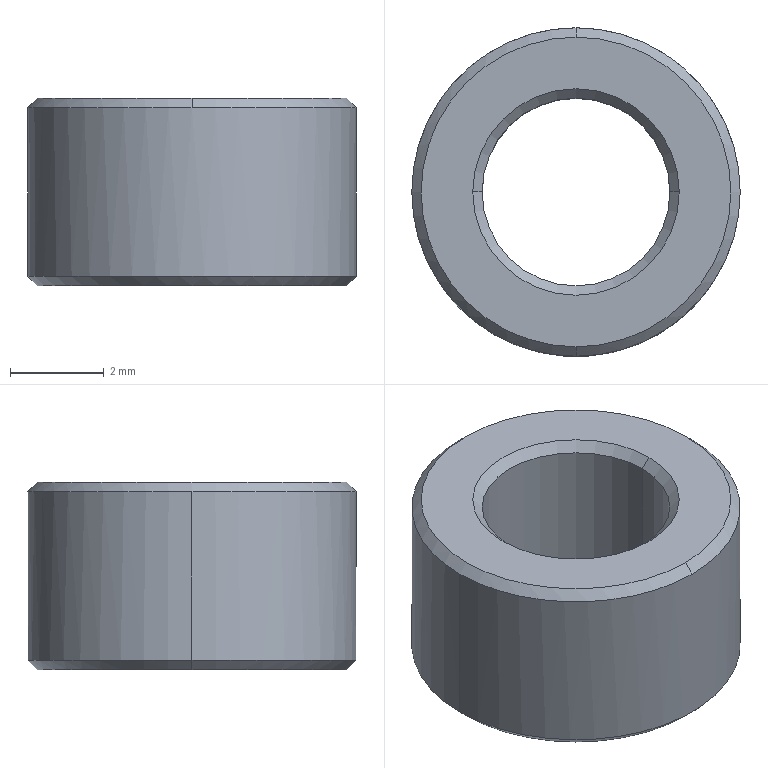Part | STEP file | 0243_001_FWSSM-D7-V4-T4 | 1 solid | 14 faces | box 7 x 7 x 4 mm | volume 102.29 mm3 | cone 8 | cylinder 4 | plane 2 | commonest cylinder face diameters 4 x2 7 x2
STEP:
#1=CARTESIAN_POINT('',(0.,0.,0.));
#2=DIRECTION('',(0.,0.,1.));
#3=DIRECTION('',(1.,0.,0.));
#4=AXIS2_PLACEMENT_3D('',#1,#2,#3);
#5=CARTESIAN_POINT('',(3.5,0.,-3.8));
#6=VERTEX_POINT('',#5);
#7=CARTESIAN_POINT('',(-3.5,0.,-3.8));
#8=VERTEX_POINT('',#7);
#9=CARTESIAN_POINT('',(0.,0.,-3.8));
#10=DIRECTION('',(0.,0.,1.));
#11=DIRECTION('',(1.,0.,0.));
#12=AXIS2_PLACEMENT_3D('',#9,#10,#11);
#13=CIRCLE('',#12,3.5);
#14=CARTESIAN_POINT('',(0.,0.,-2.));
#15=DIRECTION('',(0.,0.,1.));
#16=DIRECTION('',(1.,0.,0.));
#17=AXIS2_PLACEMENT_3D('',#14,#15,#16);
#18=CYLINDRICAL_SURFACE('',#17,3.5);
#19=CARTESIAN_POINT('',(0.,-1.8));
#20=DIRECTION('',(1.,0.));
#21=VECTOR('',#20,1.);
#22=LINE('',#19,#21);
#23=(GEOMETRIC_REPRESENTATION_CONTEXT(2)PARAMETRIC_REPRESENTATION_CONTEXT()REPRESENTATION_CONTEXT('',''));
#24=DEFINITIONAL_REPRESENTATION('',(#22),#23);
#25=PCURVE('',#18,#24);
#26=CARTESIAN_POINT('',(0.,0.,-3.8));
#27=DIRECTION('',(0.,0.,1.));
#28=DIRECTION('',(1.,0.,0.));
#29=AXIS2_PLACEMENT_3D('',#26,#27,#28);
#30=CONICAL_SURFACE('',#29,3.5,0.7854);
#31=CARTESIAN_POINT('',(0.,0.));
#32=DIRECTION('',(1.,0.));
#33=VECTOR('',#32,1.);
#34=LINE('',#31,#33);
#35=(GEOMETRIC_REPRESENTATION_CONTEXT(2)PARAMETRIC_REPRESENTATION_CONTEXT()REPRESENTATION_CONTEXT('',''));
#36=DEFINITIONAL_REPRESENTATION('',(#34),#35);
#37=PCURVE('',#30,#36);
#38=SURFACE_CURVE('',#13,(#25,#37),.PCURVE_S1.);
#39=EDGE_CURVE('',#6,#8,#38,.T.);
#40=ORIENTED_EDGE('',*,*,#39,.T.);
#41=CARTESIAN_POINT('',(-3.5,0.,-0.2));
#42=VERTEX_POINT('',#41);
#43=CARTESIAN_POINT('',(-3.5,0.,-2.));
#44=DIRECTION('',(0.,0.,1.));
#45=VECTOR('',#44,1.);
#46=LINE('',#43,#45);
#47=CARTESIAN_POINT('',(3.142,0.));
#48=DIRECTION('',(0.,1.));
#49=VECTOR('',#48,1.);
#50=LINE('',#47,#49);
#51=(GEOMETRIC_REPRESENTATION_CONTEXT(2)PARAMETRIC_REPRESENTATION_CONTEXT()REPRESENTATION_CONTEXT('',''));
#52=DEFINITIONAL_REPRESENTATION('',(#50),#51);
#53=PCURVE('',#18,#52);
#54=CARTESIAN_POINT('',(0.,0.,-2.));
#55=DIRECTION('',(0.,0.,1.));
#56=DIRECTION('',(1.,0.,0.));
#57=AXIS2_PLACEMENT_3D('',#54,#55,#56);
#58=CYLINDRICAL_SURFACE('',#57,3.5);
#59=CARTESIAN_POINT('',(3.142,0.));
#60=DIRECTION('',(0.,1.));
#61=VECTOR('',#60,1.);
#62=LINE('',#59,#61);
#63=(GEOMETRIC_REPRESENTATION_CONTEXT(2)PARAMETRIC_REPRESENTATION_CONTEXT()REPRESENTATION_CONTEXT('',''));
#64=DEFINITIONAL_REPRESENTATION('',(#62),#63);
#65=PCURVE('',#58,#64);
#66=SURFACE_CURVE('',#46,(#53,#65),.PCURVE_S1.);
#67=EDGE_CURVE('',#8,#42,#66,.T.);
#68=ORIENTED_EDGE('',*,*,#67,.T.);
#69=CARTESIAN_POINT('',(0.,3.5,-0.2));
#70=VERTEX_POINT('',#69);
#71=CARTESIAN_POINT('',(0.,0.,-0.2));
#72=DIRECTION('',(0.,0.,-1.));
#73=DIRECTION('',(1.,0.,0.));
#74=AXIS2_PLACEMENT_3D('',#71,#72,#73);
#75=CIRCLE('',#74,3.5);
#76=CARTESIAN_POINT('',(6.283,1.8));
#77=DIRECTION('',(-1.,0.));
#78=VECTOR('',#77,1.);
#79=LINE('',#76,#78);
#80=(GEOMETRIC_REPRESENTATION_CONTEXT(2)PARAMETRIC_REPRESENTATION_CONTEXT()REPRESENTATION_CONTEXT('',''));
#81=DEFINITIONAL_REPRESENTATION('',(#79),#80);
#82=PCURVE('',#18,#81);
#83=CARTESIAN_POINT('',(0.,0.,-0.2));
#84=DIRECTION('',(0.,0.,-1.));
#85=DIRECTION('',(0.,1.,0.));
#86=AXIS2_PLACEMENT_3D('',#83,#84,#85);
#87=CONICAL_SURFACE('',#86,3.5,0.7854);
#88=CARTESIAN_POINT('',(1.571,0.));
#89=DIRECTION('',(1.,0.));
#90=VECTOR('',#89,1.);
#91=LINE('',#88,#90);
#92=(GEOMETRIC_REPRESENTATION_CONTEXT(2)PARAMETRIC_REPRESENTATION_CONTEXT()REPRESENTATION_CONTEXT('',''));
#93=DEFINITIONAL_REPRESENTATION('',(#91),#92);
#94=PCURVE('',#87,#93);
#95=SURFACE_CURVE('',#75,(#82,#94),.PCURVE_S1.);
#96=EDGE_CURVE('',#42,#70,#95,.T.);
#97=ORIENTED_EDGE('',*,*,#96,.T.);
#98=CARTESIAN_POINT('',(3.5,0.,-0.2));
#99=VERTEX_POINT('',#98);
#100=CARTESIAN_POINT('',(0.,0.,-0.2));
#101=DIRECTION('',(0.,0.,-1.));
#102=DIRECTION('',(1.,0.,0.));
#103=AXIS2_PLACEMENT_3D('',#100,#101,#102);
#104=CIRCLE('',#103,3.5);
#105=CARTESIAN_POINT('',(6.283,1.8));
#106=DIRECTION('',(-1.,0.));
#107=VECTOR('',#106,1.);
#108=LINE('',#105,#107);
#109=(GEOMETRIC_REPRESENTATION_CONTEXT(2)PARAMETRIC_REPRESENTATION_CONTEXT()REPRESENTATION_CONTEXT('',''));
#110=DEFINITIONAL_REPRESENTATION('',(#108),#109);
#111=PCURVE('',#18,#110);
#112=CARTESIAN_POINT('',(0.,0.,-0.2));
#113=DIRECTION('',(0.,0.,-1.));
#114=DIRECTION('',(0.,1.,0.));
#115=AXIS2_PLACEMENT_3D('',#112,#113,#114);
#116=CONICAL_SURFACE('',#115,3.5,0.7854);
#117=CARTESIAN_POINT('',(-4.712,0.));
#118=DIRECTION('',(1.,0.));
#119=VECTOR('',#118,1.);
#120=LINE('',#117,#119);
#121=(GEOMETRIC_REPRESENTATION_CONTEXT(2)PARAMETRIC_REPRESENTATION_CONTEXT()REPRESENTATION_CONTEXT('',''));
#122=DEFINITIONAL_REPRESENTATION('',(#120),#121);
#123=PCURVE('',#116,#122);
#124=SURFACE_CURVE('',#104,(#111,#123),.PCURVE_S1.);
#125=EDGE_CURVE('',#70,#99,#124,.T.);
#126=ORIENTED_EDGE('',*,*,#125,.T.);
#127=CARTESIAN_POINT('',(3.5,0.,-2.));
#128=DIRECTION('',(0.,0.,1.));
#129=VECTOR('',#128,1.);
#130=LINE('',#127,#129);
#131=CARTESIAN_POINT('',(0.,0.));
#132=DIRECTION('',(0.,1.));
#133=VECTOR('',#132,1.);
#134=LINE('',#131,#133);
#135=(GEOMETRIC_REPRESENTATION_CONTEXT(2)PARAMETRIC_REPRESENTATION_CONTEXT()REPRESENTATION_CONTEXT('',''));
#136=DEFINITIONAL_REPRESENTATION('',(#134),#135);
#137=PCURVE('',#18,#136);
#138=CARTESIAN_POINT('',(6.283,0.));
#139=DIRECTION('',(0.,1.));
#140=VECTOR('',#139,1.);
#141=LINE('',#138,#140);
#142=(GEOMETRIC_REPRESENTATION_CONTEXT(2)PARAMETRIC_REPRESENTATION_CONTEXT()REPRESENTATION_CONTEXT('',''));
#143=DEFINITIONAL_REPRESENTATION('',(#141),#142);
#144=PCURVE('',#58,#143);
#145=SURFACE_CURVE('',#130,(#137,#144),.PCURVE_S1.);
#146=EDGE_CURVE('',#6,#99,#145,.T.);
#147=ORIENTED_EDGE('',*,*,#146,.F.);
#148=EDGE_LOOP('',(#40,#68,#97,#126,#147));
#149=FACE_BOUND('',#148,.T.);
#150=ADVANCED_FACE('',(#149),#18,.T.);
#151=CARTESIAN_POINT('',(3.3,0.,-4.));
#152=VERTEX_POINT('',#151);
#153=CARTESIAN_POINT('',(-3.3,0.,-4.));
#154=VERTEX_POINT('',#153);
#155=CARTESIAN_POINT('',(0.,0.,-4.));
#156=DIRECTION('',(0.,0.,1.));
#157=DIRECTION('',(1.,0.,0.));
#158=AXIS2_PLACEMENT_3D('',#155,#156,#157);
#159=CIRCLE('',#158,3.3);
#160=CARTESIAN_POINT('',(0.,-0.2));
#161=DIRECTION('',(1.,0.));
#162=VECTOR('',#161,1.);
#163=LINE('',#160,#162);
#164=(GEOMETRIC_REPRESENTATION_CONTEXT(2)PARAMETRIC_REPRESENTATION_CONTEXT()REPRESENTATION_CONTEXT('',''));
#165=DEFINITIONAL_REPRESENTATION('',(#163),#164);
#166=PCURVE('',#30,#165);
#167=CARTESIAN_POINT('',(1.65,0.,-4.));
#168=DIRECTION('',(0.,0.,-1.));
#169=DIRECTION('',(-1.,0.,0.));
#170=AXIS2_PLACEMENT_3D('',#167,#168,#169);
#171=PLANE('',#170);
#172=CARTESIAN_POINT('',(-1.65,0.));
#173=CARTESIAN_POINT('',(-1.65,5.716));
#174=CARTESIAN_POINT('',(3.3,2.858));
#175=CARTESIAN_POINT('',(8.25,0.));
#176=CARTESIAN_POINT('',(3.3,-2.858));
#177=CARTESIAN_POINT('',(-1.65,-5.716));
#178=CARTESIAN_POINT('',(-1.65,0.));
#179=(BOUNDED_CURVE()B_SPLINE_CURVE(2,(#172,#173,#174,#175,#176,#177,#178),.UNSPECIFIED.,.T.,.F.)B_SPLINE_CURVE_WITH_KNOTS((1,2,2,2,2,1),(-2.094,0.,2.094,4.189,6.283,8.378),.UNSPECIFIED.)CURVE()GEOMETRIC_REPRESENTATION_ITEM()RATIONAL_B_SPLINE_CURVE((1.,0.5,1.,0.5,1.,0.5,1.))REPRESENTATION_ITEM(''));
#180=(GEOMETRIC_REPRESENTATION_CONTEXT(2)PARAMETRIC_REPRESENTATION_CONTEXT()REPRESENTATION_CONTEXT('',''));
#181=DEFINITIONAL_REPRESENTATION('',(#179),#180);
#182=PCURVE('',#171,#181);
#183=SURFACE_CURVE('',#159,(#166,#182),.PCURVE_S1.);
#184=EDGE_CURVE('',#152,#154,#183,.T.);
#185=ORIENTED_EDGE('',*,*,#184,.T.);
#186=CARTESIAN_POINT('',(-3.5,0.,-3.8));
#187=DIRECTION('',(-0.7071,0.,0.7071));
#188=VECTOR('',#187,1.);
#189=LINE('',#186,#188);
#190=CARTESIAN_POINT('',(3.142,0.));
#191=DIRECTION('',(0.,1.));
#192=VECTOR('',#191,1.);
#193=LINE('',#190,#192);
#194=(GEOMETRIC_REPRESENTATION_CONTEXT(2)PARAMETRIC_REPRESENTATION_CONTEXT()REPRESENTATION_CONTEXT('',''));
#195=DEFINITIONAL_REPRESENTATION('',(#193),#194);
#196=PCURVE('',#30,#195);
#197=CARTESIAN_POINT('',(0.,0.,-3.8));
#198=DIRECTION('',(0.,0.,1.));
#199=DIRECTION('',(1.,0.,0.));
#200=AXIS2_PLACEMENT_3D('',#197,#198,#199);
#201=CONICAL_SURFACE('',#200,3.5,0.7854);
#202=CARTESIAN_POINT('',(3.142,0.));
#203=DIRECTION('',(0.,1.));
#204=VECTOR('',#203,1.);
#205=LINE('',#202,#204);
#206=(GEOMETRIC_REPRESENTATION_CONTEXT(2)PARAMETRIC_REPRESENTATION_CONTEXT()REPRESENTATION_CONTEXT('',''));
#207=DEFINITIONAL_REPRESENTATION('',(#205),#206);
#208=PCURVE('',#201,#207);
#209=SURFACE_CURVE('',#189,(#196,#208),.PCURVE_S1.);
#210=EDGE_CURVE('',#154,#8,#209,.T.);
#211=ORIENTED_EDGE('',*,*,#210,.T.);
#212=ORIENTED_EDGE('',*,*,#39,.F.);
#213=CARTESIAN_POINT('',(3.5,0.,-3.8));
#214=DIRECTION('',(0.7071,0.,0.7071));
#215=VECTOR('',#214,1.);
#216=LINE('',#213,#215);
#217=CARTESIAN_POINT('',(0.,0.));
#218=DIRECTION('',(0.,1.));
#219=VECTOR('',#218,1.);
#220=LINE('',#217,#219);
#221=(GEOMETRIC_REPRESENTATION_CONTEXT(2)PARAMETRIC_REPRESENTATION_CONTEXT()REPRESENTATION_CONTEXT('',''));
#222=DEFINITIONAL_REPRESENTATION('',(#220),#221);
#223=PCURVE('',#30,#222);
#224=CARTESIAN_POINT('',(6.283,0.));
#225=DIRECTION('',(0.,1.));
#226=VECTOR('',#225,1.);
#227=LINE('',#224,#226);
#228=(GEOMETRIC_REPRESENTATION_CONTEXT(2)PARAMETRIC_REPRESENTATION_CONTEXT()REPRESENTATION_CONTEXT('',''));
#229=DEFINITIONAL_REPRESENTATION('',(#227),#228);
#230=PCURVE('',#201,#229);
#231=SURFACE_CURVE('',#216,(#223,#230),.PCURVE_S1.);
#232=EDGE_CURVE('',#152,#6,#231,.T.);
#233=ORIENTED_EDGE('',*,*,#232,.F.);
#234=EDGE_LOOP('',(#185,#211,#212,#233));
#235=FACE_BOUND('',#234,.T.);
#236=ADVANCED_FACE('',(#235),#30,.T.);
#237=CARTESIAN_POINT('',(0.,3.3,0.));
#238=VERTEX_POINT('',#237);
#239=CARTESIAN_POINT('',(0.,-3.3,0.));
#240=VERTEX_POINT('',#239);
#241=CARTESIAN_POINT('',(0.,0.,0.));
#242=DIRECTION('',(0.,0.,-1.));
#243=DIRECTION('',(0.,1.,0.));
#244=AXIS2_PLACEMENT_3D('',#241,#242,#243);
#245=CIRCLE('',#244,3.3);
#246=CARTESIAN_POINT('',(0.,-0.2));
#247=DIRECTION('',(1.,0.));
#248=VECTOR('',#247,1.);
#249=LINE('',#246,#248);
#250=(GEOMETRIC_REPRESENTATION_CONTEXT(2)PARAMETRIC_REPRESENTATION_CONTEXT()REPRESENTATION_CONTEXT('',''));
#251=DEFINITIONAL_REPRESENTATION('',(#249),#250);
#252=PCURVE('',#116,#251);
#253=CARTESIAN_POINT('',(1.65,0.,0.));
#254=DIRECTION('',(0.,0.,1.));
#255=DIRECTION('',(1.,0.,0.));
#256=AXIS2_PLACEMENT_3D('',#253,#254,#255);
#257=PLANE('',#256);
#258=CARTESIAN_POINT('',(-1.65,3.3));
#259=CARTESIAN_POINT('',(4.066,3.3));
#260=CARTESIAN_POINT('',(1.208,-1.65));
#261=CARTESIAN_POINT('',(-1.65,-6.6));
#262=CARTESIAN_POINT('',(-4.508,-1.65));
#263=CARTESIAN_POINT('',(-7.366,3.3));
#264=CARTESIAN_POINT('',(-1.65,3.3));
#265=(BOUNDED_CURVE()B_SPLINE_CURVE(2,(#258,#259,#260,#261,#262,#263,#264),.UNSPECIFIED.,.T.,.F.)B_SPLINE_CURVE_WITH_KNOTS((1,2,2,2,2,1),(-2.094,0.,2.094,4.189,6.283,8.378),.UNSPECIFIED.)CURVE()GEOMETRIC_REPRESENTATION_ITEM()RATIONAL_B_SPLINE_CURVE((1.,0.5,1.,0.5,1.,0.5,1.))REPRESENTATION_ITEM(''));
#266=(GEOMETRIC_REPRESENTATION_CONTEXT(2)PARAMETRIC_REPRESENTATION_CONTEXT()REPRESENTATION_CONTEXT('',''));
#267=DEFINITIONAL_REPRESENTATION('',(#265),#266);
#268=PCURVE('',#257,#267);
#269=SURFACE_CURVE('',#245,(#252,#268),.PCURVE_S1.);
#270=EDGE_CURVE('',#238,#240,#269,.T.);
#271=ORIENTED_EDGE('',*,*,#270,.T.);
#272=CARTESIAN_POINT('',(0.,-3.5,-0.2));
#273=VERTEX_POINT('',#272);
#274=CARTESIAN_POINT('',(0.,-3.5,-0.2));
#275=DIRECTION('',(0.,-0.7071,-0.7071));
#276=VECTOR('',#275,1.);
#277=LINE('',#274,#276);
#278=CARTESIAN_POINT('',(3.142,0.));
#279=DIRECTION('',(0.,1.));
#280=VECTOR('',#279,1.);
#281=LINE('',#278,#280);
#282=(GEOMETRIC_REPRESENTATION_CONTEXT(2)PARAMETRIC_REPRESENTATION_CONTEXT()REPRESENTATION_CONTEXT('',''));
#283=DEFINITIONAL_REPRESENTATION('',(#281),#282);
#284=PCURVE('',#116,#283);
#285=CARTESIAN_POINT('',(3.142,0.));
#286=DIRECTION('',(0.,1.));
#287=VECTOR('',#286,1.);
#288=LINE('',#285,#287);
#289=(GEOMETRIC_REPRESENTATION_CONTEXT(2)PARAMETRIC_REPRESENTATION_CONTEXT()REPRESENTATION_CONTEXT('',''));
#290=DEFINITIONAL_REPRESENTATION('',(#288),#289);
#291=PCURVE('',#87,#290);
#292=SURFACE_CURVE('',#277,(#284,#291),.PCURVE_S1.);
#293=EDGE_CURVE('',#240,#273,#292,.T.);
#294=ORIENTED_EDGE('',*,*,#293,.T.);
#295=CARTESIAN_POINT('',(0.,0.,-0.2));
#296=DIRECTION('',(0.,0.,-1.));
#297=DIRECTION('',(1.,0.,0.));
#298=AXIS2_PLACEMENT_3D('',#295,#296,#297);
#299=CIRCLE('',#298,3.5);
#300=CARTESIAN_POINT('',(1.571,0.));
#301=DIRECTION('',(1.,0.));
#302=VECTOR('',#301,1.);
#303=LINE('',#300,#302);
#304=(GEOMETRIC_REPRESENTATION_CONTEXT(2)PARAMETRIC_REPRESENTATION_CONTEXT()REPRESENTATION_CONTEXT('',''));
#305=DEFINITIONAL_REPRESENTATION('',(#303),#304);
#306=PCURVE('',#116,#305);
#307=CARTESIAN_POINT('',(6.283,1.8));
#308=DIRECTION('',(-1.,0.));
#309=VECTOR('',#308,1.);
#310=LINE('',#307,#309);
#311=(GEOMETRIC_REPRESENTATION_CONTEXT(2)PARAMETRIC_REPRESENTATION_CONTEXT()REPRESENTATION_CONTEXT('',''));
#312=DEFINITIONAL_REPRESENTATION('',(#310),#311);
#313=PCURVE('',#58,#312);
#314=SURFACE_CURVE('',#299,(#306,#313),.PCURVE_S1.);
#315=EDGE_CURVE('',#99,#273,#314,.T.);
#316=ORIENTED_EDGE('',*,*,#315,.F.);
#317=ORIENTED_EDGE('',*,*,#125,.F.);
#318=CARTESIAN_POINT('',(0.,3.5,-0.2));
#319=DIRECTION('',(0.,0.7071,-0.7071));
#320=VECTOR('',#319,1.);
#321=LINE('',#318,#320);
#322=CARTESIAN_POINT('',(0.,0.));
#323=DIRECTION('',(0.,1.));
#324=VECTOR('',#323,1.);
#325=LINE('',#322,#324);
#326=(GEOMETRIC_REPRESENTATION_CONTEXT(2)PARAMETRIC_REPRESENTATION_CONTEXT()REPRESENTATION_CONTEXT('',''));
#327=DEFINITIONAL_REPRESENTATION('',(#325),#326);
#328=PCURVE('',#116,#327);
#329=CARTESIAN_POINT('',(6.283,0.));
#330=DIRECTION('',(0.,1.));
#331=VECTOR('',#330,1.);
#332=LINE('',#329,#331);
#333=(GEOMETRIC_REPRESENTATION_CONTEXT(2)PARAMETRIC_REPRESENTATION_CONTEXT()REPRESENTATION_CONTEXT('',''));
#334=DEFINITIONAL_REPRESENTATION('',(#332),#333);
#335=PCURVE('',#87,#334);
#336=SURFACE_CURVE('',#321,(#328,#335),.PCURVE_S1.);
#337=EDGE_CURVE('',#238,#70,#336,.T.);
#338=ORIENTED_EDGE('',*,*,#337,.F.);
#339=EDGE_LOOP('',(#271,#294,#316,#317,#338));
#340=FACE_BOUND('',#339,.T.);
#341=ADVANCED_FACE('',(#340),#116,.T.);
#342=CARTESIAN_POINT('',(-2.,0.,-3.8));
#343=VERTEX_POINT('',#342);
#344=CARTESIAN_POINT('',(-2.2,0.,-4.));
#345=VERTEX_POINT('',#344);
#346=CARTESIAN_POINT('',(-2.2,0.,-4.));
#347=DIRECTION('',(-0.7071,0.,-0.7071));
#348=VECTOR('',#347,1.);
#349=LINE('',#346,#348);
#350=CARTESIAN_POINT('',(0.,0.,-4.));
#351=DIRECTION('',(0.,0.,-1.));
#352=DIRECTION('',(-1.,0.,0.));
#353=AXIS2_PLACEMENT_3D('',#350,#351,#352);
#354=CONICAL_SURFACE('',#353,2.2,0.7854);
#355=CARTESIAN_POINT('',(6.283,0.));
#356=DIRECTION('',(0.,1.));
#357=VECTOR('',#356,1.);
#358=LINE('',#355,#357);
#359=(GEOMETRIC_REPRESENTATION_CONTEXT(2)PARAMETRIC_REPRESENTATION_CONTEXT()REPRESENTATION_CONTEXT('',''));
#360=DEFINITIONAL_REPRESENTATION('',(#358),#359);
#361=PCURVE('',#354,#360);
#362=CARTESIAN_POINT('',(0.,0.,-4.));
#363=DIRECTION('',(0.,0.,-1.));
#364=DIRECTION('',(-1.,0.,0.));
#365=AXIS2_PLACEMENT_3D('',#362,#363,#364);
#366=CONICAL_SURFACE('',#365,2.2,0.7854);
#367=CARTESIAN_POINT('',(0.,0.));
#368=DIRECTION('',(0.,1.));
#369=VECTOR('',#368,1.);
#370=LINE('',#367,#369);
#371=(GEOMETRIC_REPRESENTATION_CONTEXT(2)PARAMETRIC_REPRESENTATION_CONTEXT()REPRESENTATION_CONTEXT('',''));
#372=DEFINITIONAL_REPRESENTATION('',(#370),#371);
#373=PCURVE('',#366,#372);
#374=SURFACE_CURVE('',#349,(#361,#373),.PCURVE_S1.);
#375=EDGE_CURVE('',#343,#345,#374,.T.);
#376=ORIENTED_EDGE('',*,*,#375,.T.);
#377=CARTESIAN_POINT('',(2.2,0.,-4.));
#378=VERTEX_POINT('',#377);
#379=CARTESIAN_POINT('',(0.,0.,-4.));
#380=DIRECTION('',(0.,0.,1.));
#381=DIRECTION('',(-1.,0.,0.));
#382=AXIS2_PLACEMENT_3D('',#379,#380,#381);
#383=CIRCLE('',#382,2.2);
#384=CARTESIAN_POINT('',(6.283,0.));
#385=DIRECTION('',(-1.,0.));
#386=VECTOR('',#385,1.);
#387=LINE('',#384,#386);
#388=(GEOMETRIC_REPRESENTATION_CONTEXT(2)PARAMETRIC_REPRESENTATION_CONTEXT()REPRESENTATION_CONTEXT('',''));
#389=DEFINITIONAL_REPRESENTATION('',(#387),#388);
#390=PCURVE('',#354,#389);
#391=CARTESIAN_POINT('',(3.85,0.));
#392=CARTESIAN_POINT('',(3.85,-3.811));
#393=CARTESIAN_POINT('',(0.55,-1.905));
#394=CARTESIAN_POINT('',(-2.75,0.));
#395=CARTESIAN_POINT('',(0.55,1.905));
#396=CARTESIAN_POINT('',(3.85,3.811));
#397=CARTESIAN_POINT('',(3.85,0.));
#398=(BOUNDED_CURVE()B_SPLINE_CURVE(2,(#391,#392,#393,#394,#395,#396,#397),.UNSPECIFIED.,.T.,.F.)B_SPLINE_CURVE_WITH_KNOTS((1,2,2,2,2,1),(-2.094,0.,2.094,4.189,6.283,8.378),.UNSPECIFIED.)CURVE()GEOMETRIC_REPRESENTATION_ITEM()RATIONAL_B_SPLINE_CURVE((1.,0.5,1.,0.5,1.,0.5,1.))REPRESENTATION_ITEM(''));
#399=(GEOMETRIC_REPRESENTATION_CONTEXT(2)PARAMETRIC_REPRESENTATION_CONTEXT()REPRESENTATION_CONTEXT('',''));
#400=DEFINITIONAL_REPRESENTATION('',(#398),#399);
#401=PCURVE('',#171,#400);
#402=SURFACE_CURVE('',#383,(#390,#401),.PCURVE_S1.);
#403=EDGE_CURVE('',#345,#378,#402,.T.);
#404=ORIENTED_EDGE('',*,*,#403,.T.);
#405=CARTESIAN_POINT('',(2.,0.,-3.8));
#406=VERTEX_POINT('',#405);
#407=CARTESIAN_POINT('',(2.2,0.,-4.));
#408=DIRECTION('',(0.7071,0.,-0.7071));
#409=VECTOR('',#408,1.);
#410=LINE('',#407,#409);
#411=CARTESIAN_POINT('',(3.142,0.));
#412=DIRECTION('',(0.,1.));
#413=VECTOR('',#412,1.);
#414=LINE('',#411,#413);
#415=(GEOMETRIC_REPRESENTATION_CONTEXT(2)PARAMETRIC_REPRESENTATION_CONTEXT()REPRESENTATION_CONTEXT('',''));
#416=DEFINITIONAL_REPRESENTATION('',(#414),#415);
#417=PCURVE('',#354,#416);
#418=CARTESIAN_POINT('',(3.142,0.));
#419=DIRECTION('',(0.,1.));
#420=VECTOR('',#419,1.);
#421=LINE('',#418,#420);
#422=(GEOMETRIC_REPRESENTATION_CONTEXT(2)PARAMETRIC_REPRESENTATION_CONTEXT()REPRESENTATION_CONTEXT('',''));
#423=DEFINITIONAL_REPRESENTATION('',(#421),#422);
#424=PCURVE('',#366,#423);
#425=SURFACE_CURVE('',#410,(#417,#424),.PCURVE_S1.);
#426=EDGE_CURVE('',#406,#378,#425,.T.);
#427=ORIENTED_EDGE('',*,*,#426,.F.);
#428=CARTESIAN_POINT('',(0.,0.,-3.8));
#429=DIRECTION('',(0.,0.,-1.));
#430=DIRECTION('',(1.,0.,0.));
#431=AXIS2_PLACEMENT_3D('',#428,#429,#430);
#432=CIRCLE('',#431,2.);
#433=CARTESIAN_POINT('',(3.142,-0.2));
#434=DIRECTION('',(1.,0.));
#435=VECTOR('',#434,1.);
#436=LINE('',#433,#435);
#437=(GEOMETRIC_REPRESENTATION_CONTEXT(2)PARAMETRIC_REPRESENTATION_CONTEXT()REPRESENTATION_CONTEXT('',''));
#438=DEFINITIONAL_REPRESENTATION('',(#436),#437);
#439=PCURVE('',#354,#438);
#440=CARTESIAN_POINT('',(0.,0.,-2.));
#441=DIRECTION('',(0.,0.,1.));
#442=DIRECTION('',(1.,0.,0.));
#443=AXIS2_PLACEMENT_3D('',#440,#441,#442);
#444=CYLINDRICAL_SURFACE('',#443,2.);
#445=CARTESIAN_POINT('',(6.283,-1.8));
#446=DIRECTION('',(-1.,0.));
#447=VECTOR('',#446,1.);
#448=LINE('',#445,#447);
#449=(GEOMETRIC_REPRESENTATION_CONTEXT(2)PARAMETRIC_REPRESENTATION_CONTEXT()REPRESENTATION_CONTEXT('',''));
#450=DEFINITIONAL_REPRESENTATION('',(#448),#449);
#451=PCURVE('',#444,#450);
#452=SURFACE_CURVE('',#432,(#439,#451),.PCURVE_S1.);
#453=EDGE_CURVE('',#406,#343,#452,.T.);
#454=ORIENTED_EDGE('',*,*,#453,.T.);
#455=EDGE_LOOP('',(#376,#404,#427,#454));
#456=FACE_BOUND('',#455,.F.);
#457=ADVANCED_FACE('',(#456),#354,.F.);
#458=CARTESIAN_POINT('',(2.,0.,-0.2));
#459=VERTEX_POINT('',#458);
#460=CARTESIAN_POINT('',(2.2,0.,0.));
#461=VERTEX_POINT('',#460);
#462=CARTESIAN_POINT('',(2.2,0.,0.));
#463=DIRECTION('',(0.7071,0.,0.7071));
#464=VECTOR('',#463,1.);
#465=LINE('',#462,#464);
#466=CARTESIAN_POINT('',(0.,0.,0.));
#467=DIRECTION('',(0.,0.,1.));
#468=DIRECTION('',(1.,0.,0.));
#469=AXIS2_PLACEMENT_3D('',#466,#467,#468);
#470=CONICAL_SURFACE('',#469,2.2,0.7854);
#471=CARTESIAN_POINT('',(6.283,0.));
#472=DIRECTION('',(0.,1.));
#473=VECTOR('',#472,1.);
#474=LINE('',#471,#473);
#475=(GEOMETRIC_REPRESENTATION_CONTEXT(2)PARAMETRIC_REPRESENTATION_CONTEXT()REPRESENTATION_CONTEXT('',''));
#476=DEFINITIONAL_REPRESENTATION('',(#474),#475);
#477=PCURVE('',#470,#476);
#478=CARTESIAN_POINT('',(0.,0.,0.));
#479=DIRECTION('',(0.,0.,1.));
#480=DIRECTION('',(1.,0.,0.));
#481=AXIS2_PLACEMENT_3D('',#478,#479,#480);
#482=CONICAL_SURFACE('',#481,2.2,0.7854);
#483=CARTESIAN_POINT('',(0.,0.));
#484=DIRECTION('',(0.,1.));
#485=VECTOR('',#484,1.);
#486=LINE('',#483,#485);
#487=(GEOMETRIC_REPRESENTATION_CONTEXT(2)PARAMETRIC_REPRESENTATION_CONTEXT()REPRESENTATION_CONTEXT('',''));
#488=DEFINITIONAL_REPRESENTATION('',(#486),#487);
#489=PCURVE('',#482,#488);
#490=SURFACE_CURVE('',#465,(#477,#489),.PCURVE_S1.);
#491=EDGE_CURVE('',#459,#461,#490,.T.);
#492=ORIENTED_EDGE('',*,*,#491,.T.);
#493=CARTESIAN_POINT('',(-2.2,0.,0.));
#494=VERTEX_POINT('',#493);
#495=CARTESIAN_POINT('',(0.,0.,0.));
#496=DIRECTION('',(0.,0.,-1.));
#497=DIRECTION('',(1.,0.,0.));
#498=AXIS2_PLACEMENT_3D('',#495,#496,#497);
#499=CIRCLE('',#498,2.2);
#500=CARTESIAN_POINT('',(6.283,0.));
#501=DIRECTION('',(-1.,0.));
#502=VECTOR('',#501,1.);
#503=LINE('',#500,#502);
#504=(GEOMETRIC_REPRESENTATION_CONTEXT(2)PARAMETRIC_REPRESENTATION_CONTEXT()REPRESENTATION_CONTEXT('',''));
#505=DEFINITIONAL_REPRESENTATION('',(#503),#504);
#506=PCURVE('',#470,#505);
#507=CARTESIAN_POINT('',(0.55,0.));
#508=CARTESIAN_POINT('',(0.55,-3.811));
#509=CARTESIAN_POINT('',(-2.75,-1.905));
#510=CARTESIAN_POINT('',(-6.05,0.));
#511=CARTESIAN_POINT('',(-2.75,1.905));
#512=CARTESIAN_POINT('',(0.55,3.811));
#513=CARTESIAN_POINT('',(0.55,0.));
#514=(BOUNDED_CURVE()B_SPLINE_CURVE(2,(#507,#508,#509,#510,#511,#512,#513),.UNSPECIFIED.,.T.,.F.)B_SPLINE_CURVE_WITH_KNOTS((1,2,2,2,2,1),(-2.094,0.,2.094,4.189,6.283,8.378),.UNSPECIFIED.)CURVE()GEOMETRIC_REPRESENTATION_ITEM()RATIONAL_B_SPLINE_CURVE((1.,0.5,1.,0.5,1.,0.5,1.))REPRESENTATION_ITEM(''));
#515=(GEOMETRIC_REPRESENTATION_CONTEXT(2)PARAMETRIC_REPRESENTATION_CONTEXT()REPRESENTATION_CONTEXT('',''));
#516=DEFINITIONAL_REPRESENTATION('',(#514),#515);
#517=PCURVE('',#257,#516);
#518=SURFACE_CURVE('',#499,(#506,#517),.PCURVE_S1.);
#519=EDGE_CURVE('',#461,#494,#518,.T.);
#520=ORIENTED_EDGE('',*,*,#519,.T.);
#521=CARTESIAN_POINT('',(-2.,0.,-0.2));
#522=VERTEX_POINT('',#521);
#523=CARTESIAN_POINT('',(-2.2,0.,0.));
#524=DIRECTION('',(-0.7071,0.,0.7071));
#525=VECTOR('',#524,1.);
#526=LINE('',#523,#525);
#527=CARTESIAN_POINT('',(3.142,0.));
#528=DIRECTION('',(0.,1.));
#529=VECTOR('',#528,1.);
#530=LINE('',#527,#529);
#531=(GEOMETRIC_REPRESENTATION_CONTEXT(2)PARAMETRIC_REPRESENTATION_CONTEXT()REPRESENTATION_CONTEXT('',''));
#532=DEFINITIONAL_REPRESENTATION('',(#530),#531);
#533=PCURVE('',#470,#532);
#534=CARTESIAN_POINT('',(3.142,0.));
#535=DIRECTION('',(0.,1.));
#536=VECTOR('',#535,1.);
#537=LINE('',#534,#536);
#538=(GEOMETRIC_REPRESENTATION_CONTEXT(2)PARAMETRIC_REPRESENTATION_CONTEXT()REPRESENTATION_CONTEXT('',''));
#539=DEFINITIONAL_REPRESENTATION('',(#537),#538);
#540=PCURVE('',#482,#539);
#541=SURFACE_CURVE('',#526,(#533,#540),.PCURVE_S1.);
#542=EDGE_CURVE('',#522,#494,#541,.T.);
#543=ORIENTED_EDGE('',*,*,#542,.F.);
#544=CARTESIAN_POINT('',(0.,0.,-0.2));
#545=DIRECTION('',(0.,0.,1.));
#546=DIRECTION('',(1.,0.,0.));
#547=AXIS2_PLACEMENT_3D('',#544,#545,#546);
#548=CIRCLE('',#547,2.);
#549=CARTESIAN_POINT('',(0.,-0.2));
#550=DIRECTION('',(1.,0.));
#551=VECTOR('',#550,1.);
#552=LINE('',#549,#551);
#553=(GEOMETRIC_REPRESENTATION_CONTEXT(2)PARAMETRIC_REPRESENTATION_CONTEXT()REPRESENTATION_CONTEXT('',''));
#554=DEFINITIONAL_REPRESENTATION('',(#552),#553);
#555=PCURVE('',#470,#554);
#556=CARTESIAN_POINT('',(0.,1.8));
#557=DIRECTION('',(1.,0.));
#558=VECTOR('',#557,1.);
#559=LINE('',#556,#558);
#560=(GEOMETRIC_REPRESENTATION_CONTEXT(2)PARAMETRIC_REPRESENTATION_CONTEXT()REPRESENTATION_CONTEXT('',''));
#561=DEFINITIONAL_REPRESENTATION('',(#559),#560);
#562=PCURVE('',#444,#561);
#563=SURFACE_CURVE('',#548,(#555,#562),.PCURVE_S1.);
#564=EDGE_CURVE('',#522,#459,#563,.T.);
#565=ORIENTED_EDGE('',*,*,#564,.T.);
#566=EDGE_LOOP('',(#492,#520,#543,#565));
#567=FACE_BOUND('',#566,.F.);
#568=ADVANCED_FACE('',(#567),#470,.F.);
#569=CARTESIAN_POINT('',(2.,0.,-2.));
#570=DIRECTION('',(0.,0.,1.));
#571=VECTOR('',#570,1.);
#572=LINE('',#569,#571);
#573=CARTESIAN_POINT('',(6.283,0.));
#574=DIRECTION('',(0.,1.));
#575=VECTOR('',#574,1.);
#576=LINE('',#573,#575);
#577=(GEOMETRIC_REPRESENTATION_CONTEXT(2)PARAMETRIC_REPRESENTATION_CONTEXT()REPRESENTATION_CONTEXT('',''));
#578=DEFINITIONAL_REPRESENTATION('',(#576),#577);
#579=PCURVE('',#444,#578);
#580=CARTESIAN_POINT('',(0.,0.,-2.));
#581=DIRECTION('',(0.,0.,1.));
#582=DIRECTION('',(1.,0.,0.));
#583=AXIS2_PLACEMENT_3D('',#580,#581,#582);
#584=CYLINDRICAL_SURFACE('',#583,2.);
#585=CARTESIAN_POINT('',(0.,0.));
#586=DIRECTION('',(0.,1.));
#587=VECTOR('',#586,1.);
#588=LINE('',#585,#587);
#589=(GEOMETRIC_REPRESENTATION_CONTEXT(2)PARAMETRIC_REPRESENTATION_CONTEXT()REPRESENTATION_CONTEXT('',''));
#590=DEFINITIONAL_REPRESENTATION('',(#588),#589);
#591=PCURVE('',#584,#590);
#592=SURFACE_CURVE('',#572,(#579,#591),.PCURVE_S1.);
#593=EDGE_CURVE('',#406,#459,#592,.T.);
#594=ORIENTED_EDGE('',*,*,#593,.T.);
#595=ORIENTED_EDGE('',*,*,#564,.F.);
#596=CARTESIAN_POINT('',(-2.,0.,-2.));
#597=DIRECTION('',(0.,0.,1.));
#598=VECTOR('',#597,1.);
#599=LINE('',#596,#598);
#600=CARTESIAN_POINT('',(3.142,0.));
#601=DIRECTION('',(0.,1.));
#602=VECTOR('',#601,1.);
#603=LINE('',#600,#602);
#604=(GEOMETRIC_REPRESENTATION_CONTEXT(2)PARAMETRIC_REPRESENTATION_CONTEXT()REPRESENTATION_CONTEXT('',''));
#605=DEFINITIONAL_REPRESENTATION('',(#603),#604);
#606=PCURVE('',#444,#605);
#607=CARTESIAN_POINT('',(3.142,0.));
#608=DIRECTION('',(0.,1.));
#609=VECTOR('',#608,1.);
#610=LINE('',#607,#609);
#611=(GEOMETRIC_REPRESENTATION_CONTEXT(2)PARAMETRIC_REPRESENTATION_CONTEXT()REPRESENTATION_CONTEXT('',''));
#612=DEFINITIONAL_REPRESENTATION('',(#610),#611);
#613=PCURVE('',#584,#612);
#614=SURFACE_CURVE('',#599,(#606,#613),.PCURVE_S1.);
#615=EDGE_CURVE('',#343,#522,#614,.T.);
#616=ORIENTED_EDGE('',*,*,#615,.F.);
#617=ORIENTED_EDGE('',*,*,#453,.F.);
#618=EDGE_LOOP('',(#594,#595,#616,#617));
#619=FACE_BOUND('',#618,.F.);
#620=ADVANCED_FACE('',(#619),#444,.F.);
#621=ORIENTED_EDGE('',*,*,#67,.F.);
#622=CARTESIAN_POINT('',(0.,0.,-3.8));
#623=DIRECTION('',(0.,0.,1.));
#624=DIRECTION('',(1.,0.,0.));
#625=AXIS2_PLACEMENT_3D('',#622,#623,#624);
#626=CIRCLE('',#625,3.5);
#627=CARTESIAN_POINT('',(0.,-1.8));
#628=DIRECTION('',(1.,0.));
#629=VECTOR('',#628,1.);
#630=LINE('',#627,#629);
#631=(GEOMETRIC_REPRESENTATION_CONTEXT(2)PARAMETRIC_REPRESENTATION_CONTEXT()REPRESENTATION_CONTEXT('',''));
#632=DEFINITIONAL_REPRESENTATION('',(#630),#631);
#633=PCURVE('',#58,#632);
#634=CARTESIAN_POINT('',(0.,0.));
#635=DIRECTION('',(1.,0.));
#636=VECTOR('',#635,1.);
#637=LINE('',#634,#636);
#638=(GEOMETRIC_REPRESENTATION_CONTEXT(2)PARAMETRIC_REPRESENTATION_CONTEXT()REPRESENTATION_CONTEXT('',''));
#639=DEFINITIONAL_REPRESENTATION('',(#637),#638);
#640=PCURVE('',#201,#639);
#641=SURFACE_CURVE('',#626,(#633,#640),.PCURVE_S1.);
#642=EDGE_CURVE('',#8,#6,#641,.T.);
#643=ORIENTED_EDGE('',*,*,#642,.T.);
#644=ORIENTED_EDGE('',*,*,#146,.T.);
#645=ORIENTED_EDGE('',*,*,#315,.T.);
#646=CARTESIAN_POINT('',(0.,0.,-0.2));
#647=DIRECTION('',(0.,0.,-1.));
#648=DIRECTION('',(1.,0.,0.));
#649=AXIS2_PLACEMENT_3D('',#646,#647,#648);
#650=CIRCLE('',#649,3.5);
#651=CARTESIAN_POINT('',(6.283,1.8));
#652=DIRECTION('',(-1.,0.));
#653=VECTOR('',#652,1.);
#654=LINE('',#651,#653);
#655=(GEOMETRIC_REPRESENTATION_CONTEXT(2)PARAMETRIC_REPRESENTATION_CONTEXT()REPRESENTATION_CONTEXT('',''));
#656=DEFINITIONAL_REPRESENTATION('',(#654),#655);
#657=PCURVE('',#58,#656);
#658=CARTESIAN_POINT('',(1.571,0.));
#659=DIRECTION('',(1.,0.));
#660=VECTOR('',#659,1.);
#661=LINE('',#658,#660);
#662=(GEOMETRIC_REPRESENTATION_CONTEXT(2)PARAMETRIC_REPRESENTATION_CONTEXT()REPRESENTATION_CONTEXT('',''));
#663=DEFINITIONAL_REPRESENTATION('',(#661),#662);
#664=PCURVE('',#87,#663);
#665=SURFACE_CURVE('',#650,(#657,#664),.PCURVE_S1.);
#666=EDGE_CURVE('',#273,#42,#665,.T.);
#667=ORIENTED_EDGE('',*,*,#666,.T.);
#668=EDGE_LOOP('',(#621,#643,#644,#645,#667));
#669=FACE_BOUND('',#668,.T.);
#670=ADVANCED_FACE('',(#669),#58,.T.);
#671=ORIENTED_EDGE('',*,*,#210,.F.);
#672=CARTESIAN_POINT('',(0.,0.,-4.));
#673=DIRECTION('',(0.,0.,1.));
#674=DIRECTION('',(1.,0.,0.));
#675=AXIS2_PLACEMENT_3D('',#672,#673,#674);
#676=CIRCLE('',#675,3.3);
#677=CARTESIAN_POINT('',(0.,-0.2));
#678=DIRECTION('',(1.,0.));
#679=VECTOR('',#678,1.);
#680=LINE('',#677,#679);
#681=(GEOMETRIC_REPRESENTATION_CONTEXT(2)PARAMETRIC_REPRESENTATION_CONTEXT()REPRESENTATION_CONTEXT('',''));
#682=DEFINITIONAL_REPRESENTATION('',(#680),#681);
#683=PCURVE('',#201,#682);
#684=CARTESIAN_POINT('',(-1.65,0.));
#685=CARTESIAN_POINT('',(-1.65,5.716));
#686=CARTESIAN_POINT('',(3.3,2.858));
#687=CARTESIAN_POINT('',(8.25,0.));
#688=CARTESIAN_POINT('',(3.3,-2.858));
#689=CARTESIAN_POINT('',(-1.65,-5.716));
#690=CARTESIAN_POINT('',(-1.65,0.));
#691=(BOUNDED_CURVE()B_SPLINE_CURVE(2,(#684,#685,#686,#687,#688,#689,#690),.UNSPECIFIED.,.T.,.F.)B_SPLINE_CURVE_WITH_KNOTS((1,2,2,2,2,1),(-2.094,0.,2.094,4.189,6.283,8.378),.UNSPECIFIED.)CURVE()GEOMETRIC_REPRESENTATION_ITEM()RATIONAL_B_SPLINE_CURVE((1.,0.5,1.,0.5,1.,0.5,1.))REPRESENTATION_ITEM(''));
#692=(GEOMETRIC_REPRESENTATION_CONTEXT(2)PARAMETRIC_REPRESENTATION_CONTEXT()REPRESENTATION_CONTEXT('',''));
#693=DEFINITIONAL_REPRESENTATION('',(#691),#692);
#694=PCURVE('',#171,#693);
#695=SURFACE_CURVE('',#676,(#683,#694),.PCURVE_S1.);
#696=EDGE_CURVE('',#154,#152,#695,.T.);
#697=ORIENTED_EDGE('',*,*,#696,.T.);
#698=ORIENTED_EDGE('',*,*,#232,.T.);
#699=ORIENTED_EDGE('',*,*,#642,.F.);
#700=EDGE_LOOP('',(#671,#697,#698,#699));
#701=FACE_BOUND('',#700,.T.);
#702=ADVANCED_FACE('',(#701),#201,.T.);
#703=ORIENTED_EDGE('',*,*,#293,.F.);
#704=CARTESIAN_POINT('',(0.,0.,0.));
#705=DIRECTION('',(0.,0.,-1.));
#706=DIRECTION('',(0.,1.,0.));
#707=AXIS2_PLACEMENT_3D('',#704,#705,#706);
#708=CIRCLE('',#707,3.3);
#709=CARTESIAN_POINT('',(0.,-0.2));
#710=DIRECTION('',(1.,0.));
#711=VECTOR('',#710,1.);
#712=LINE('',#709,#711);
#713=(GEOMETRIC_REPRESENTATION_CONTEXT(2)PARAMETRIC_REPRESENTATION_CONTEXT()REPRESENTATION_CONTEXT('',''));
#714=DEFINITIONAL_REPRESENTATION('',(#712),#713);
#715=PCURVE('',#87,#714);
#716=CARTESIAN_POINT('',(-1.65,3.3));
#717=CARTESIAN_POINT('',(4.066,3.3));
#718=CARTESIAN_POINT('',(1.208,-1.65));
#719=CARTESIAN_POINT('',(-1.65,-6.6));
#720=CARTESIAN_POINT('',(-4.508,-1.65));
#721=CARTESIAN_POINT('',(-7.366,3.3));
#722=CARTESIAN_POINT('',(-1.65,3.3));
#723=(BOUNDED_CURVE()B_SPLINE_CURVE(2,(#716,#717,#718,#719,#720,#721,#722),.UNSPECIFIED.,.T.,.F.)B_SPLINE_CURVE_WITH_KNOTS((1,2,2,2,2,1),(-2.094,0.,2.094,4.189,6.283,8.378),.UNSPECIFIED.)CURVE()GEOMETRIC_REPRESENTATION_ITEM()RATIONAL_B_SPLINE_CURVE((1.,0.5,1.,0.5,1.,0.5,1.))REPRESENTATION_ITEM(''));
#724=(GEOMETRIC_REPRESENTATION_CONTEXT(2)PARAMETRIC_REPRESENTATION_CONTEXT()REPRESENTATION_CONTEXT('',''));
#725=DEFINITIONAL_REPRESENTATION('',(#723),#724);
#726=PCURVE('',#257,#725);
#727=SURFACE_CURVE('',#708,(#715,#726),.PCURVE_S1.);
#728=EDGE_CURVE('',#240,#238,#727,.T.);
#729=ORIENTED_EDGE('',*,*,#728,.T.);
#730=ORIENTED_EDGE('',*,*,#337,.T.);
#731=ORIENTED_EDGE('',*,*,#96,.F.);
#732=ORIENTED_EDGE('',*,*,#666,.F.);
#733=EDGE_LOOP('',(#703,#729,#730,#731,#732));
#734=FACE_BOUND('',#733,.T.);
#735=ADVANCED_FACE('',(#734),#87,.T.);
#736=ORIENTED_EDGE('',*,*,#184,.F.);
#737=ORIENTED_EDGE('',*,*,#696,.F.);
#738=EDGE_LOOP('',(#736,#737));
#739=FACE_BOUND('',#738,.T.);
#740=ORIENTED_EDGE('',*,*,#403,.T.);
#741=CARTESIAN_POINT('',(0.,0.,-4.));
#742=DIRECTION('',(0.,0.,1.));
#743=DIRECTION('',(-1.,0.,0.));
#744=AXIS2_PLACEMENT_3D('',#741,#742,#743);
#745=CIRCLE('',#744,2.2);
#746=CARTESIAN_POINT('',(3.85,0.));
#747=CARTESIAN_POINT('',(3.85,-3.811));
#748=CARTESIAN_POINT('',(0.55,-1.905));
#749=CARTESIAN_POINT('',(-2.75,0.));
#750=CARTESIAN_POINT('',(0.55,1.905));
#751=CARTESIAN_POINT('',(3.85,3.811));
#752=CARTESIAN_POINT('',(3.85,0.));
#753=(BOUNDED_CURVE()B_SPLINE_CURVE(2,(#746,#747,#748,#749,#750,#751,#752),.UNSPECIFIED.,.T.,.F.)B_SPLINE_CURVE_WITH_KNOTS((1,2,2,2,2,1),(-2.094,0.,2.094,4.189,6.283,8.378),.UNSPECIFIED.)CURVE()GEOMETRIC_REPRESENTATION_ITEM()RATIONAL_B_SPLINE_CURVE((1.,0.5,1.,0.5,1.,0.5,1.))REPRESENTATION_ITEM(''));
#754=(GEOMETRIC_REPRESENTATION_CONTEXT(2)PARAMETRIC_REPRESENTATION_CONTEXT()REPRESENTATION_CONTEXT('',''));
#755=DEFINITIONAL_REPRESENTATION('',(#753),#754);
#756=PCURVE('',#171,#755);
#757=CARTESIAN_POINT('',(6.283,0.));
#758=DIRECTION('',(-1.,0.));
#759=VECTOR('',#758,1.);
#760=LINE('',#757,#759);
#761=(GEOMETRIC_REPRESENTATION_CONTEXT(2)PARAMETRIC_REPRESENTATION_CONTEXT()REPRESENTATION_CONTEXT('',''));
#762=DEFINITIONAL_REPRESENTATION('',(#760),#761);
#763=PCURVE('',#366,#762);
#764=SURFACE_CURVE('',#745,(#756,#763),.PCURVE_S1.);
#765=EDGE_CURVE('',#378,#345,#764,.T.);
#766=ORIENTED_EDGE('',*,*,#765,.T.);
#767=EDGE_LOOP('',(#740,#766));
#768=FACE_BOUND('',#767,.T.);
#769=ADVANCED_FACE('',(#739,#768),#171,.T.);
#770=ORIENTED_EDGE('',*,*,#270,.F.);
#771=ORIENTED_EDGE('',*,*,#728,.F.);
#772=EDGE_LOOP('',(#770,#771));
#773=FACE_BOUND('',#772,.T.);
#774=ORIENTED_EDGE('',*,*,#519,.T.);
#775=CARTESIAN_POINT('',(0.,0.,0.));
#776=DIRECTION('',(0.,0.,-1.));
#777=DIRECTION('',(1.,0.,0.));
#778=AXIS2_PLACEMENT_3D('',#775,#776,#777);
#779=CIRCLE('',#778,2.2);
#780=CARTESIAN_POINT('',(0.55,0.));
#781=CARTESIAN_POINT('',(0.55,-3.811));
#782=CARTESIAN_POINT('',(-2.75,-1.905));
#783=CARTESIAN_POINT('',(-6.05,0.));
#784=CARTESIAN_POINT('',(-2.75,1.905));
#785=CARTESIAN_POINT('',(0.55,3.811));
#786=CARTESIAN_POINT('',(0.55,0.));
#787=(BOUNDED_CURVE()B_SPLINE_CURVE(2,(#780,#781,#782,#783,#784,#785,#786),.UNSPECIFIED.,.T.,.F.)B_SPLINE_CURVE_WITH_KNOTS((1,2,2,2,2,1),(-2.094,0.,2.094,4.189,6.283,8.378),.UNSPECIFIED.)CURVE()GEOMETRIC_REPRESENTATION_ITEM()RATIONAL_B_SPLINE_CURVE((1.,0.5,1.,0.5,1.,0.5,1.))REPRESENTATION_ITEM(''));
#788=(GEOMETRIC_REPRESENTATION_CONTEXT(2)PARAMETRIC_REPRESENTATION_CONTEXT()REPRESENTATION_CONTEXT('',''));
#789=DEFINITIONAL_REPRESENTATION('',(#787),#788);
#790=PCURVE('',#257,#789);
#791=CARTESIAN_POINT('',(6.283,0.));
#792=DIRECTION('',(-1.,0.));
#793=VECTOR('',#792,1.);
#794=LINE('',#791,#793);
#795=(GEOMETRIC_REPRESENTATION_CONTEXT(2)PARAMETRIC_REPRESENTATION_CONTEXT()REPRESENTATION_CONTEXT('',''));
#796=DEFINITIONAL_REPRESENTATION('',(#794),#795);
#797=PCURVE('',#482,#796);
#798=SURFACE_CURVE('',#779,(#790,#797),.PCURVE_S1.);
#799=EDGE_CURVE('',#494,#461,#798,.T.);
#800=ORIENTED_EDGE('',*,*,#799,.T.);
#801=EDGE_LOOP('',(#774,#800));
#802=FACE_BOUND('',#801,.T.);
#803=ADVANCED_FACE('',(#773,#802),#257,.T.);
#804=ORIENTED_EDGE('',*,*,#765,.T.);
#805=ORIENTED_EDGE('',*,*,#375,.F.);
#806=CARTESIAN_POINT('',(0.,0.,-3.8));
#807=DIRECTION('',(0.,0.,-1.));
#808=DIRECTION('',(1.,0.,0.));
#809=AXIS2_PLACEMENT_3D('',#806,#807,#808);
#810=CIRCLE('',#809,2.);
#811=CARTESIAN_POINT('',(-3.142,-0.2));
#812=DIRECTION('',(1.,0.));
#813=VECTOR('',#812,1.);
#814=LINE('',#811,#813);
#815=(GEOMETRIC_REPRESENTATION_CONTEXT(2)PARAMETRIC_REPRESENTATION_CONTEXT()REPRESENTATION_CONTEXT('',''));
#816=DEFINITIONAL_REPRESENTATION('',(#814),#815);
#817=PCURVE('',#366,#816);
#818=CARTESIAN_POINT('',(6.283,-1.8));
#819=DIRECTION('',(-1.,0.));
#820=VECTOR('',#819,1.);
#821=LINE('',#818,#820);
#822=(GEOMETRIC_REPRESENTATION_CONTEXT(2)PARAMETRIC_REPRESENTATION_CONTEXT()REPRESENTATION_CONTEXT('',''));
#823=DEFINITIONAL_REPRESENTATION('',(#821),#822);
#824=PCURVE('',#584,#823);
#825=SURFACE_CURVE('',#810,(#817,#824),.PCURVE_S1.);
#826=EDGE_CURVE('',#343,#406,#825,.T.);
#827=ORIENTED_EDGE('',*,*,#826,.T.);
#828=ORIENTED_EDGE('',*,*,#426,.T.);
#829=EDGE_LOOP('',(#804,#805,#827,#828));
#830=FACE_BOUND('',#829,.F.);
#831=ADVANCED_FACE('',(#830),#366,.F.);
#832=ORIENTED_EDGE('',*,*,#799,.T.);
#833=ORIENTED_EDGE('',*,*,#491,.F.);
#834=CARTESIAN_POINT('',(0.,0.,-0.2));
#835=DIRECTION('',(0.,0.,1.));
#836=DIRECTION('',(1.,0.,0.));
#837=AXIS2_PLACEMENT_3D('',#834,#835,#836);
#838=CIRCLE('',#837,2.);
#839=CARTESIAN_POINT('',(0.,-0.2));
#840=DIRECTION('',(1.,0.));
#841=VECTOR('',#840,1.);
#842=LINE('',#839,#841);
#843=(GEOMETRIC_REPRESENTATION_CONTEXT(2)PARAMETRIC_REPRESENTATION_CONTEXT()REPRESENTATION_CONTEXT('',''));
#844=DEFINITIONAL_REPRESENTATION('',(#842),#843);
#845=PCURVE('',#482,#844);
#846=CARTESIAN_POINT('',(0.,1.8));
#847=DIRECTION('',(1.,0.));
#848=VECTOR('',#847,1.);
#849=LINE('',#846,#848);
#850=(GEOMETRIC_REPRESENTATION_CONTEXT(2)PARAMETRIC_REPRESENTATION_CONTEXT()REPRESENTATION_CONTEXT('',''));
#851=DEFINITIONAL_REPRESENTATION('',(#849),#850);
#852=PCURVE('',#584,#851);
#853=SURFACE_CURVE('',#838,(#845,#852),.PCURVE_S1.);
#854=EDGE_CURVE('',#459,#522,#853,.T.);
#855=ORIENTED_EDGE('',*,*,#854,.T.);
#856=ORIENTED_EDGE('',*,*,#542,.T.);
#857=EDGE_LOOP('',(#832,#833,#855,#856));
#858=FACE_BOUND('',#857,.F.);
#859=ADVANCED_FACE('',(#858),#482,.F.);
#860=ORIENTED_EDGE('',*,*,#854,.F.);
#861=ORIENTED_EDGE('',*,*,#593,.F.);
#862=ORIENTED_EDGE('',*,*,#826,.F.);
#863=ORIENTED_EDGE('',*,*,#615,.T.);
#864=EDGE_LOOP('',(#860,#861,#862,#863));
#865=FACE_BOUND('',#864,.F.);
#866=ADVANCED_FACE('',(#865),#584,.F.);
#867=CLOSED_SHELL('',(#150,#236,#341,#457,#568,#620,#670,#702,#735,#769,#803,#831,#859,#866));
#868=MANIFOLD_SOLID_BREP('',#867);
#869=(LENGTH_UNIT()NAMED_UNIT(*)SI_UNIT(.MILLI.,.METRE.));
#870=UNCERTAINTY_MEASURE_WITH_UNIT(LENGTH_MEASURE(0.0000001),#869,'','');
#871=(NAMED_UNIT(*)PLANE_ANGLE_UNIT()SI_UNIT($,.RADIAN.));
#872=(NAMED_UNIT(*)SI_UNIT($,.STERADIAN.)SOLID_ANGLE_UNIT());
#873=(GEOMETRIC_REPRESENTATION_CONTEXT(3)GLOBAL_UNCERTAINTY_ASSIGNED_CONTEXT((#870))GLOBAL_UNIT_ASSIGNED_CONTEXT((#869,#871,#872))REPRESENTATION_CONTEXT('',''));
#874=ADVANCED_BREP_SHAPE_REPRESENTATION('',(#4,#868),#873);